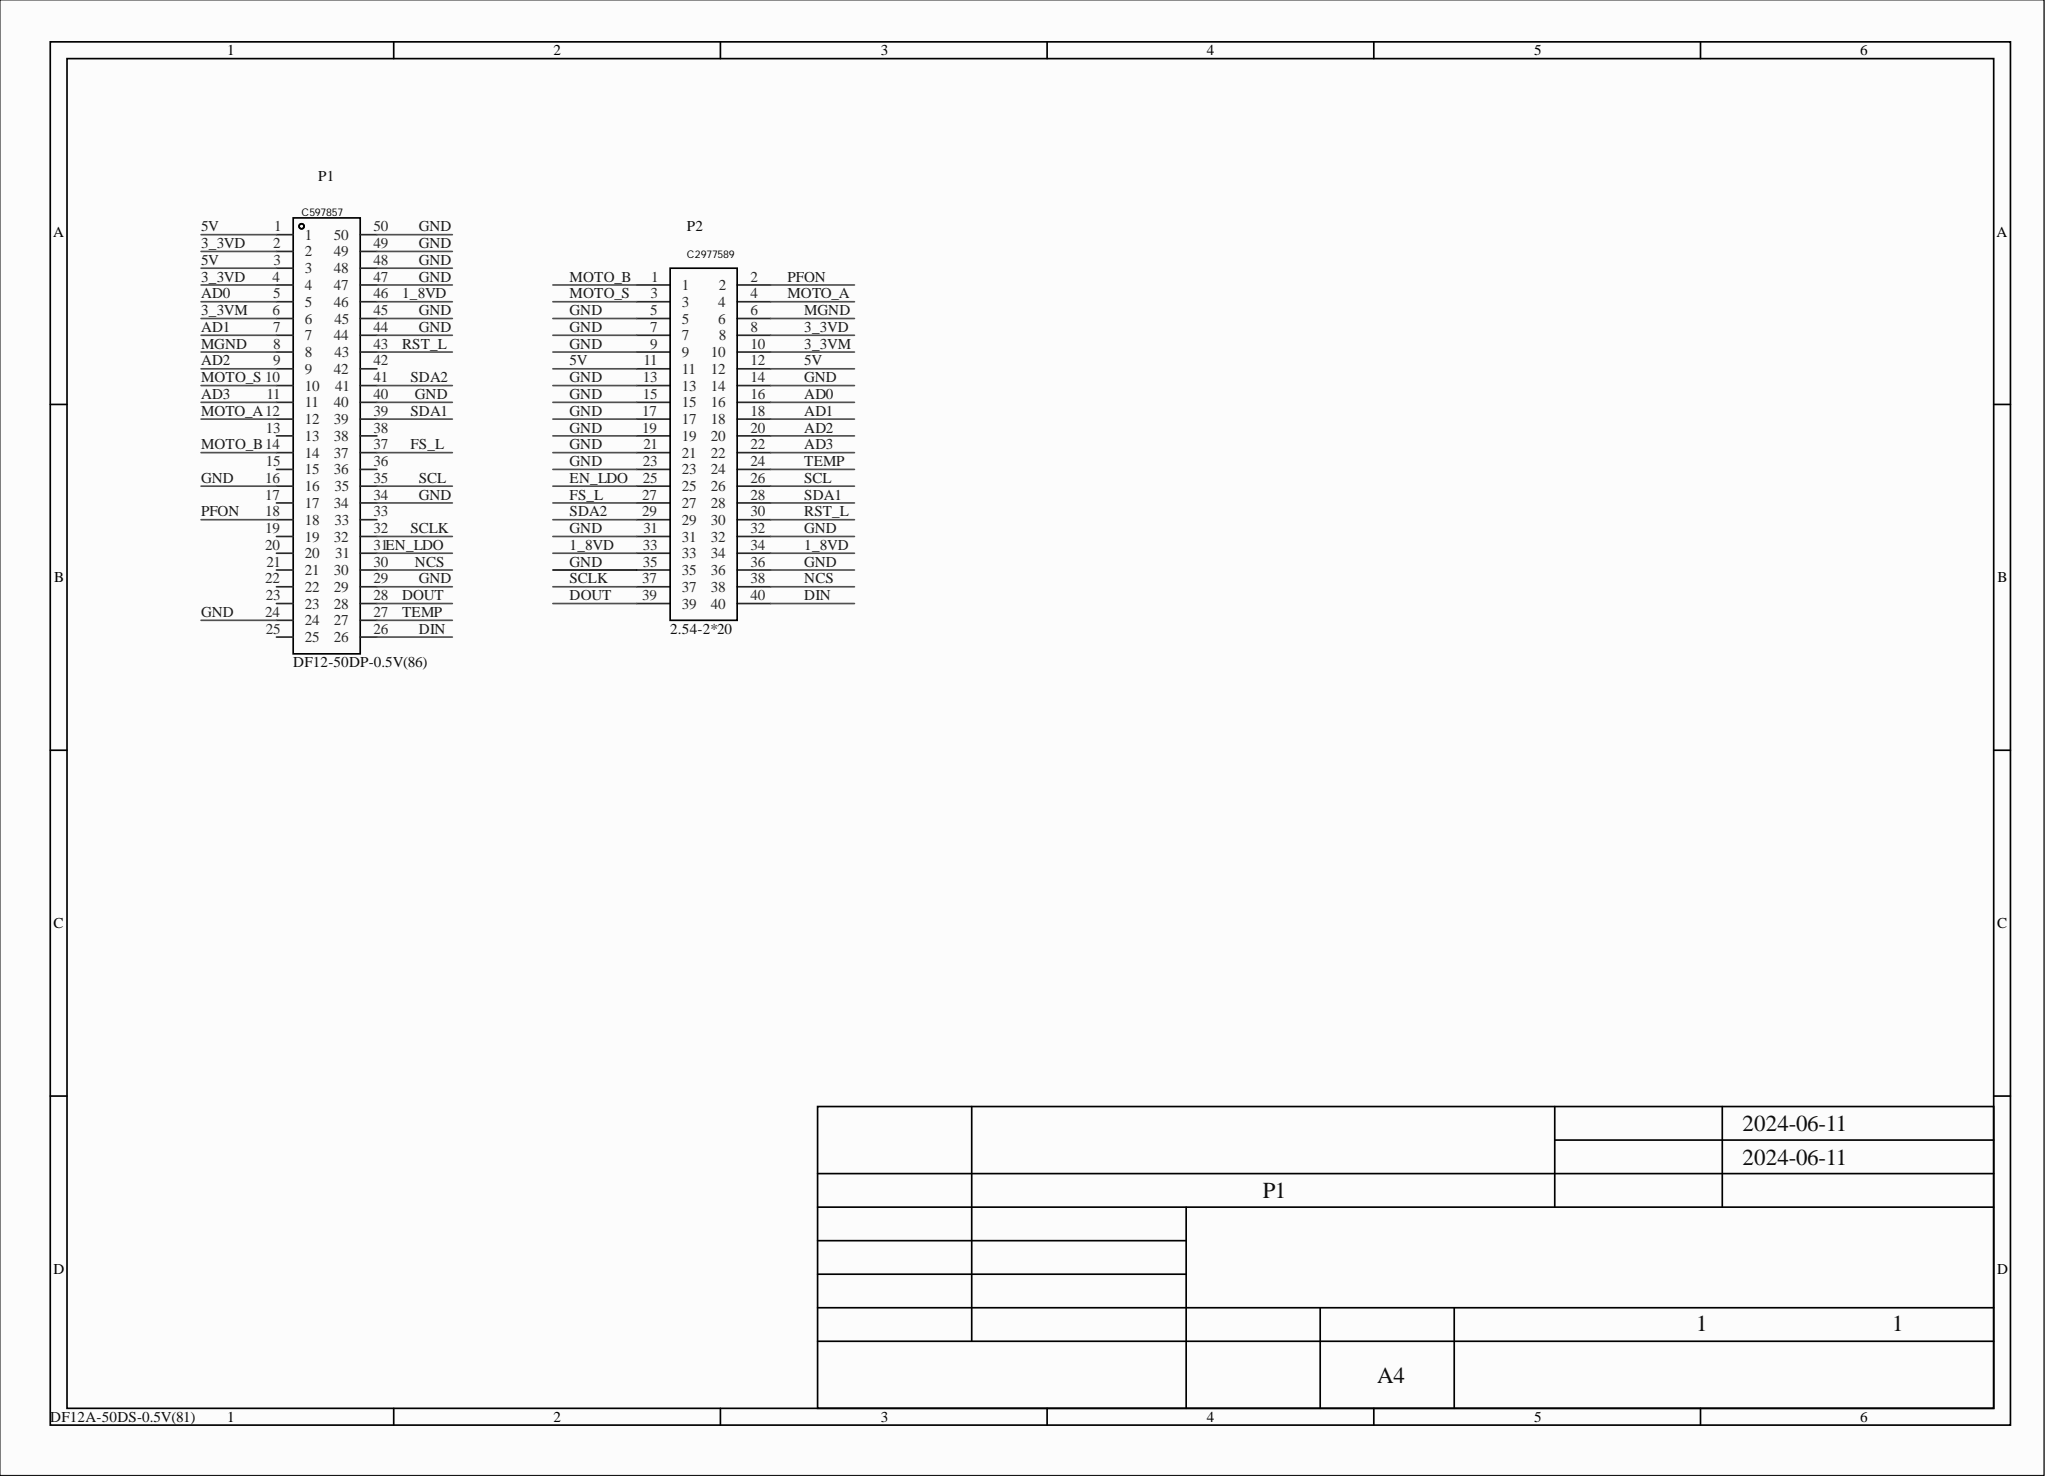Circuit board | Altium Designer | 2 parts | 25 nets
Bill of materials:
Comment,Description,Designator,Footprint,LibRef,Quantity
"DF12A-50DS-0.5V(81)","","P1","CONN-SMD_DF12A-3.0-50DS-0.5","DF12A-50DS-0.5V(81)","1"
"2.54-2*20","","P2","HDR-TH_40P-P2.54-V-F-R2-C20-S2.54","2.54-2*20","1"
Netlist (Protel format):
[
P1
CONN-SMD_DF12A-3.0-50DS-0.5
DF12A-50DS-0.5V(81)



]
[
P2
HDR-TH_40P-P2.54-V-F-R2-C20-S2.54
2.54-2*20



]
(
TEMP
P1-27
P2-24
)
(
SDA2
P1-41
P2-29
)
(
SDA1
P1-39
P2-28
)
(
SCLK
P1-32
P2-37
)
(
SCL
P1-35
P2-26
)
(
RST_L
P1-43
P2-30
)
(
PFON
P1-18
P2-2
)
(
NCS
P1-30
P2-38
)
(
MOTO_S
P1-10
P2-3
)
(
MOTO_B
P1-14
P2-1
)
(
MOTO_A
P1-12
P2-4
)
(
MGND
P1-8
P2-6
)
(
GND
P1-16
P1-24
P1-29
P1-34
P1-40
P1-44
P1-45
P1-47
P1-48
P1-49
P1-50
P2-5
P2-7
P2-9
P2-13
P2-14
P2-15
P2-17
P2-19
P2-21
P2-23
P2-31
P2-32
P2-35
P2-36
)
(
FS_L
P1-37
P2-27
)
(
EN_LDO
P1-31
P2-25
)
(
DOUT
P1-28
P2-39
)
(
DIN
P1-26
P2-40
)
(
AD3
P1-11
P2-22
)
(
AD2
P1-9
P2-20
)
(
AD1
P1-7
P2-18
)
(
AD0
P1-5
P2-16
)
(
5V
P1-1
P1-3
P2-11
P2-12
)
(
3_3VM
P1-6
P2-10
)
(
3_3VD
P1-2
P1-4
P2-8
)
(
1_8VD
P1-46
P2-33
P2-34
)